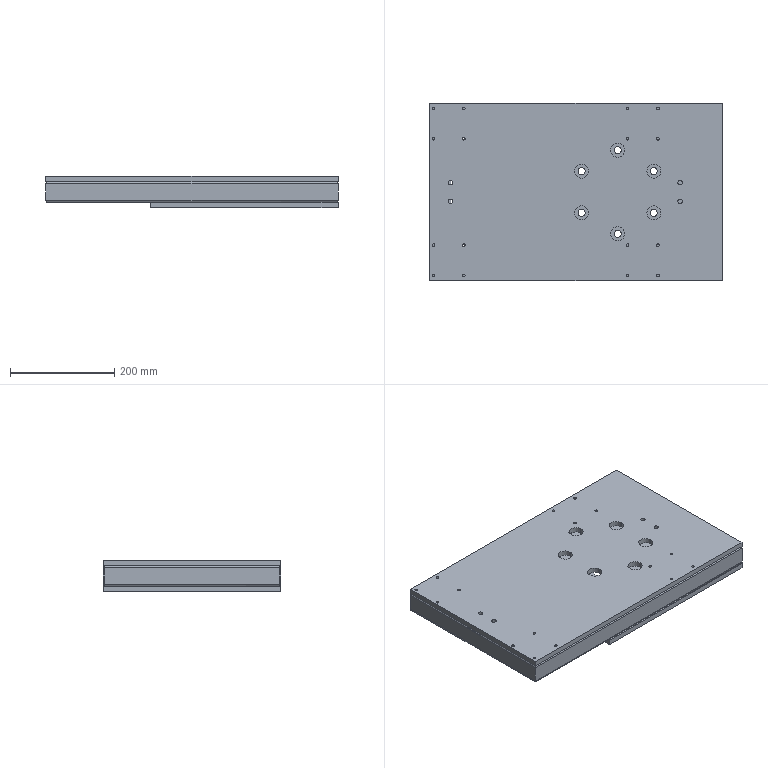Part | SolidWorks | features BaseBody 7 | 7 solids | 208 faces | box 560 x 340 x 60 mm | volume 3618040 mm3 | cylinder 132 | plane 76 | commonest cylinder face diameters 5 x56 4 x20 8 x20 13.5 x12 27 x12 8.5 x10